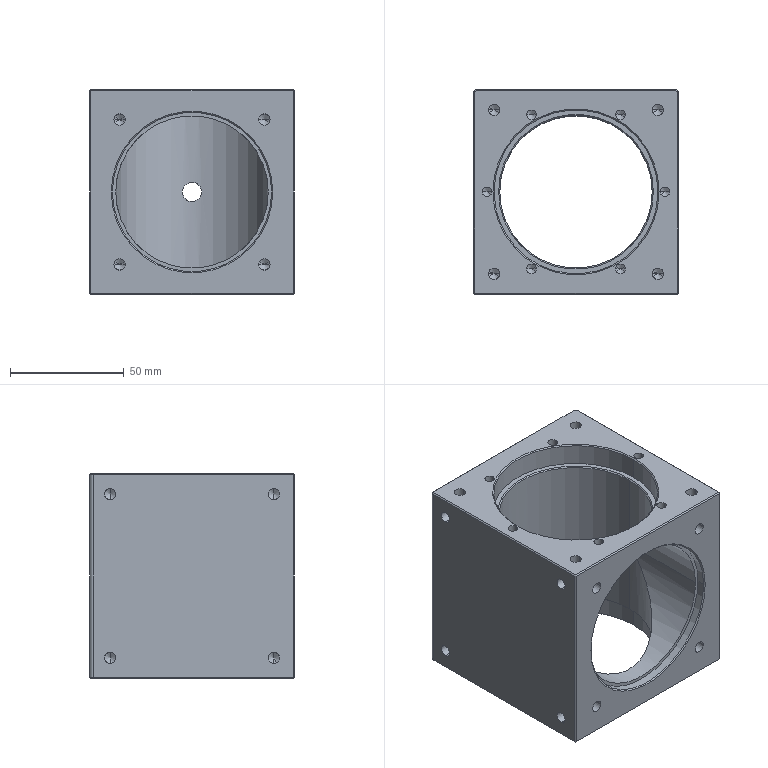NC program | NX | posted with a generic post | part box 90 x 90 x 90 mm
Whole program:
N10 G17 G21 G94 G90
(DRILLING_COPY_1_COPY_1_COPY_COPY , TOOL : D6A45)
N12 T07 M6
N14 G54
N16 G17 G0 G90 X0. Y0. B0. C0. S5000 M3
N18 G43 Z30. H7
N20 G94 G81 G98 Z-1. F250. R3.
N22 X-19.55 Y33.862
N24 X-36. Y36.
N26 X-39.1 Y0.
N28 X-36. Y-36.
N30 X-19.55 Y-33.862
N32 X19.55
N34 X36. Y-36.
N36 X39.1 Y0.
N38 X36. Y36.
N40 X19.55 Y33.862
N42 G80
N44 G0 X19.55 Y33.862 Z30.
N46 M5
(DRILLING_COPY_1_COPY_COPY_COPY_COPY_COPY_1_COPY_1 , TOOL : 5.0ZT)
N48 T15 M6
N50 G54
N52 G17 G0 G90 X-36. Y36. B0. C0. S2000 M3
N54 G43 Z30. H15
N56 G94 G83 G98 Z-10.234 F150. Q2. R3.
N58 Y-36. Z-12.002
N60 X36.
N62 Y36. Z-10.234
N64 G80
N66 G0 X36. Y36. Z30.
N68 M5
(DRILLING_COPY_1_COPY_COPY_COPY_COPY_COPY_1_COPY_COPY , TOOL : 4.2ZT)
N70 T14 M6
N72 G54
N74 G17 G0 G90 X-39.1 Y0. B0. C0. S2000 M3
N76 G43 Z30. H14
N78 G94 G83 G98 Z-15.262 F150. Q2. R3.
N80 X-19.55 Y33.862
N82 X19.55
N84 X39.1 Y0.
N86 X19.55 Y-33.862
N88 X-19.55
N90 G80
N92 G0 X-19.55 Y-33.862 Z30.
N94 M5
(DRILLING_COPY_1_COPY_COPY_COPY_COPY_COPY_COPY_COPY , TOOL : 9.0ZT)
N96 T09 M6
N98 G54
N100 G17 G0 G90 X0. Y0. B0. C0. S1200 M3
N102 G43 Z30. H9
N104 G94 G83 G98 Z-49.704 F150. Q2. R3.
N106 G80
N108 G0 X0. Y0. Z30.
N110 M5
(HOLE_MILLING_COPY_1_COPY , TOOL : D10)
N112 T10 M6
N114 G54
N116 G17 G0 G90 X0. Y0. B0. C0. S9500 M3
N118 G43 Z30. H10
N120 Z0.5
N122 G94 G3 X-1.25 Y1.25 R1.25 F2200.
N124 X-2.5 Y0. R1.25
N126 X-2.5 Y0. Z-0.5 I2.5 J0.
N128 X-2.5 Y0. Z-1.5 I2.5 J0.
N130 X-2.5 Y0. Z-2.5 I2.5 J0.
N132 X-2.5 Y0. Z-3.5 I2.5 J0.
N134 X-2.5 Y0. Z-4.5 I2.5 J0.
N136 X-2.5 Y0. Z-5.5 I2.5 J0.
N138 X-2.5 Y0. Z-6.5 I2.5 J0.
N140 X-2.5 Y0. Z-7.5 I2.5 J0.
N142 X-2.5 Y0. Z-8.5 I2.5 J0.
N144 X-2.5 Y0. Z-9.5 I2.5 J0.
N146 X0.099 Y-2.678 R2.68
N148 X2.987 Y-0.165 R2.819
N150 X0.334 Y3.217 R3.076
N152 X-3.461 Y0.383 R3.39
N154 X-0.578 Y-3.681 R3.568
N156 X3.919 Y-0.654 R3.881
N158 X0.874 Y4.126 R4.06
N160 X-4.357 Y0.976 R4.373
N162 X-1.22 Y-4.548 R4.551
N164 X4.769 Y-1.349 R4.865
N166 X1.615 Y4.943 R5.043
N168 X-5.152 Y1.769 R5.356
N170 X-2.058 Y-5.307 R5.534
N172 X5.502 Y-2.235 R5.847
N174 X2.544 Y5.635 R6.025
N176 X-5.815 Y2.744 R6.339
N178 X-3.072 Y-5.925 R6.517
N180 X6.087 Y-3.294 R6.83
N182 X3.64 Y6.172 R7.008
N184 X-6.315 Y3.882 R7.322
N186 X-4.243 Y-6.374 R7.5
N188 X6.495 Y-4.503 R7.813
N190 X4.879 Y6.526 R7.991
N192 X-6.625 Y5.156 R8.304
N194 X-5.543 Y-6.627 R8.482
N196 X6.701 Y-5.836 R8.796
N198 X6.232 Y6.673 R8.974
N200 X-6.721 Y6.539 R9.287
N202 X-6.943 Y-6.662 R9.465
N204 X6.684 Y-7.26 R9.778
N206 X7.67 Y6.592 R9.956
N208 X-6.586 Y7.997 R10.269
N210 X-8.409 Y-6.461 R10.447
N212 X6.426 Y-8.743 R10.761
N214 X9.156 Y6.268 R10.939
N216 X-6.204 Y9.495 R11.252
N218 X-9.906 Y-6.012 R11.43
N220 X5.917 Y-10.248 R11.743
N222 X10.654 Y5.691 R11.921
N224 X-5.565 Y10.997 R12.235
N226 X-11.395 Y-5.305 R12.413
N228 X5.148 Y-11.736 R12.726
N230 X12.125 Y4.854 R12.904
N232 X-4.666 Y12.462 R13.217
N234 X-12.839 Y-4.338 R13.395
N236 X4.119 Y-13.169 R13.708
N238 X13.531 Y3.758 R13.886
N240 X-3.508 Y13.852 R14.2
N242 X-14.197 Y-3.114 R14.378
N244 X2.834 Y-14.507 R14.691
N246 X14.832 Y2.408 R14.869
N248 X-2.098 Y15.127 R15.182
N250 X-15.43 Y-1.642 R15.36
N252 X1.302 Y-15.709 R15.673
N254 X15.987 Y0.816 R15.851
N256 X-0.448 Y16.248 R16.165
N258 X-16.499 Y0.066 R16.343
N260 X-0.461 Y-16.739 R16.656
N262 X16.961 Y-1.002 R16.834
N264 X1.423 Y17.178 R17.147
N266 X-17.369 Y1.989 R17.325
N268 X-2.435 Y-17.56 R17.638
N270 X17.717 Y-3.023 R17.816
N272 X3.493 Y17.881 R18.13
N274 X-18.003 Y4.102 R18.308
N276 X-4.593 Y-18.138 R18.621
N278 X18.222 Y-5.221 R18.799
N280 X5.732 Y18.326 R19.112
N282 X-18.372 Y6.377 R19.29
N284 X-6.905 Y-18.443 R19.603
N286 X18.448 Y-7.564 R19.781
N288 X8.108 Y18.484 R20.095
N290 X-18.447 Y8.778 R20.273
N292 X-9.336 Y-18.448 R20.586
N294 X18.368 Y-10.015 R20.764
N296 X10.583 Y18.331 R21.077
N298 X-18.207 Y11.269 R21.255
N300 X-11.846 Y-18.131 R21.568
N302 X17.962 Y-12.535 R21.746
N304 X13.117 Y17.847 R22.06
N306 X-17.632 Y13.807 R22.238
N308 X-14.393 Y-17.476 R22.551
N310 X17.215 Y-15.08 R22.729
N312 X15.667 Y17.018 R23.042
N314 X-16.71 Y16.348 R23.22
N316 X-16.932 Y-16.472 R23.533
N318 X16.117 Y-17.605 R23.711
N320 X18.185 Y15.837 R24.025
N322 X-15.435 Y18.845 R24.202
N324 X-19.417 Y-15.113 R24.516
N326 X14.664 Y-20.063 R24.694
N328 X20.624 Y14.3 R25.007
N330 X-13.805 Y21.251 R25.185
N332 X-21.799 Y-13.4 R25.498
N334 X12.859 Y-22.405 R25.676
N336 X22.936 Y12.412 R25.989
N338 X-11.827 Y23.518 R26.167
N340 X-24.029 Y-11.34 R26.481
N342 X10.711 Y-24.583 R26.659
N344 X25.072 Y10.183 R26.972
N346 X-9.513 Y25.596 R27.15
N348 X-26.06 Y-8.946 R27.463
N350 X8.235 Y-26.55 R27.641
N352 X26.986 Y7.631 R27.954
N354 X-6.881 Y27.44 R28.132
N356 X-27.844 Y-6.24 R28.446
N358 X5.453 Y-28.259 R28.624
N360 X28.63 Y4.778 R28.937
N362 X-3.955 Y29.003 R29.115
N364 X-29.338 Y-3.247 R29.428
N366 X2.392 Y-29.667 R29.606
N368 X29.963 Y1.653 R29.919
N370 X-1.001 Y30.316 R30.177
N372 X-30.5 Y0. R30.328
N374 X0. Y-30.5 R30.5
N376 X-30.5 Y0. R-30.5
N378 X-15.25 Y-15.25 R15.25
N380 X0. Y0. R15.25
N382 G0 Z30.
N384 M5
(HOLE_MILLING_COPY_COPY_1_COPY , TOOL : D16)
N386 T16 M6
N388 G54
N390 G17 G0 G90 X0. Y0. B0. C0. S8500 M3
N392 G43 Z30. H16
N394 Z-10.
N396 G94 G3 X1.5 Y-1.5 R1.5 F2200.
N398 X3. Y0. R1.5
N400 X3. Y0. Z-11. I-3. J0.
N402 X3. Y0. Z-12. I-3. J0.
N404 X3. Y0. Z-13. I-3. J0.
N406 X3. Y0. Z-14. I-3. J0.
N408 X3. Y0. Z-15. I-3. J0.
N410 X3. Y0. Z-16. I-3. J0.
N412 X3. Y0. Z-17. I-3. J0.
N414 X3. Y0. Z-18. I-3. J0.
N416 X3. Y0. Z-19. I-3. J0.
N418 X3. Y0. Z-20. I-3. J0.
N420 X3. Y0. Z-21. I-3. J0.
N422 X3. Y0. Z-22. I-3. J0.
N424 X3. Y0. Z-23. I-3. J0.
N426 X3. Y0. Z-24. I-3. J0.
N428 X3. Y0. Z-25. I-3. J0.
N430 X3. Y0. Z-26. I-3. J0.
N432 X3. Y0. Z-27. I-3. J0.
N434 X3. Y0. Z-28. I-3. J0.
N436 X0. Y-3. Z-28.75 R-3.
N438 X3.177 Y0.106 R3.178
N440 X0.146 Y3.49 R3.322
N442 X-3.726 Y0.302 R3.579
N444 X-0.334 Y-3.973 R3.894
N446 X4.201 Y-0.509 R4.073
N448 X0.561 Y4.445 R4.388
N450 X-4.664 Y0.756 R4.567
N452 X-0.829 Y-4.904 R4.881
N454 X5.113 Y-1.043 R5.06
N456 X1.137 Y5.347 R5.375
N458 X-5.545 Y1.369 R5.554
N460 X-1.482 Y-5.773 R5.868
N462 X5.958 Y-1.733 R6.047
N464 X1.865 Y6.178 R6.362
N466 X-6.35 Y2.133 R6.541
N468 X-2.285 Y-6.56 R6.855
N470 X6.718 Y-2.569 R7.034
N472 X2.739 Y6.918 R7.349
N474 X-7.059 Y3.04 R7.528
N476 X-3.227 Y-7.247 R7.842
N478 X7.372 Y-3.543 R8.021
N480 X3.747 Y7.548 R8.336
N482 X-7.654 Y4.077 R8.515
N484 X-4.297 Y-7.817 R8.829
N486 X7.904 Y-4.64 R9.008
N488 X4.876 Y8.052 R9.323
N490 X-8.12 Y5.232 R9.501
N492 X-5.482 Y-8.251 R9.816
N494 X8.299 Y-5.849 R9.995
N496 X6.113 Y8.414 R10.309
N498 X-8.439 Y6.489 R10.488
N500 X-6.766 Y-8.537 R10.803
N502 X8.54 Y-7.152 R10.982
N504 X7.44 Y8.62 R11.296
N506 X-8.6 Y7.833 R11.475
N508 X-8.132 Y-8.66 R11.79
N510 X8.617 Y-8.531 R11.968
N512 X8.84 Y8.657 R12.283
N514 X-8.59 Y9.244 R12.462
N516 X-9.562 Y-8.609 R12.776
N518 X8.518 Y-9.97 R12.955
N520 X10.294 Y8.516 R13.27
N522 X-8.399 Y10.704 R13.448
N524 X-11.035 Y-8.376 R13.763
N526 X8.234 Y-11.446 R13.942
N528 X11.781 Y8.188 R14.256
N530 X-8.02 Y12.191 R14.435
N532 X-12.53 Y-7.952 R14.75
N534 X7.758 Y-12.938 R14.929
N536 X13.279 Y7.667 R15.243
N538 X-7.447 Y13.684 R15.422
N540 X-14.026 Y-7.332 R15.736
N542 X7.087 Y-14.426 R15.915
N544 X14.767 Y6.949 R16.23
N546 X-6.677 Y15.161 R16.409
N548 X-15.5 Y-6.515 R16.723
N550 X6.218 Y-15.886 R16.902
N552 X16.221 Y6.033 R17.217
N554 X-5.71 Y16.598 R17.395
N556 X-16.929 Y-5.501 R17.71
N558 X5.152 Y-17.295 R17.889
N560 X17.619 Y4.919 R18.203
N562 X-4.546 Y17.974 R18.382
N564 X-18.29 Y-4.29 R18.697
N566 X3.892 Y-18.631 R18.875
N568 X18.938 Y3.613 R19.19
N570 X-3.191 Y19.264 R19.369
N572 X-19.561 Y-2.889 R19.683
N574 X2.443 Y-19.87 R19.862
N576 X20.156 Y2.118 R20.177
N578 X-1.65 Y20.446 R20.355
N580 X-20.719 Y-1.304 R20.67
N582 X0.813 Y-20.991 R20.849
N584 X21.249 Y0.445 R21.163
N586 X0.066 Y21.5 R21.342
N588 X-21.742 Y0.455 R21.657
N590 X-0.987 Y-21.971 R21.836
N592 X22.196 Y-1.396 R22.15
N594 X1.948 Y22.402 R22.329
N596 X-22.609 Y2.376 R22.643
N598 X-2.946 Y-22.79 R22.822
N600 X22.977 Y-3.393 R23.137
N602 X3.98 Y23.133 R23.316
N604 X-23.3 Y4.445 R23.63
N606 X-5.048 Y-23.429 R23.809
N608 X23.574 Y-5.529 R24.123
N610 X6.147 Y23.675 R24.302
N612 X-23.797 Y6.644 R24.617
N614 X-7.076 Y-24.012 R24.875
N616 X23.967 Y-7.787 R25.028
N618 X7.787 Y23.967 R25.2
N620 X23.967 Y-7.787 R-25.2
N622 X15.877 Y8.09 R12.6
N624 X0. Y0. R12.6
N626 X1.5 Y-1.5 R1.5
N628 X3. Y0. R1.5
N630 X3. Y0. Z-29.75 I-3. J0.
N632 X3. Y0. Z-30.75 I-3. J0.
N634 X3. Y0. Z-31.75 I-3. J0.
N636 X3. Y0. Z-32.75 I-3. J0.
N638 X3. Y0. Z-33.75 I-3. J0.
N640 X3. Y0. Z-34.75 I-3. J0.
N642 X3. Y0. Z-35.75 I-3. J0.
N644 X3. Y0. Z-36.75 I-3. J0.
N646 X3. Y0. Z-37.75 I-3. J0.
N648 X3. Y0. Z-38.75 I-3. J0.
N650 X3. Y0. Z-39.75 I-3. J0.
N652 X3. Y0. Z-40.75 I-3. J0.
N654 X3. Y0. Z-41.75 I-3. J0.
N656 X3. Y0. Z-42.75 I-3. J0.
N658 X3. Y0. Z-43.75 I-3. J0.
N660 X3. Y0. Z-44.75 I-3. J0.
N662 X3. Y0. Z-45.75 I-3. J0.
N664 X3. Y0. Z-46.75 I-3. J0.
N666 X0. Y-3. Z-47.5 R-3.
N668 X3.177 Y0.106 R3.178
N670 X0.146 Y3.49 R3.322
N672 X-3.726 Y0.302 R3.579
N674 X-0.334 Y-3.973 R3.894
N676 X4.201 Y-0.509 R4.073
N678 X0.561 Y4.445 R4.388
N680 X-4.664 Y0.756 R4.567
N682 X-0.829 Y-4.904 R4.881
N684 X5.113 Y-1.043 R5.06
N686 X1.137 Y5.347 R5.375
N688 X-5.545 Y1.369 R5.554
N690 X-1.482 Y-5.773 R5.868
N692 X5.958 Y-1.733 R6.047
N694 X1.865 Y6.178 R6.362
N696 X-6.35 Y2.133 R6.541
N698 X-2.285 Y-6.56 R6.855
N700 X6.718 Y-2.569 R7.034
N702 X2.739 Y6.918 R7.349
N704 X-7.059 Y3.04 R7.528
N706 X-3.227 Y-7.247 R7.842
N708 X7.372 Y-3.543 R8.021
N710 X3.747 Y7.548 R8.336
N712 X-7.654 Y4.077 R8.515
N714 X-4.297 Y-7.817 R8.829
N716 X7.904 Y-4.64 R9.008
N718 X4.876 Y8.052 R9.323
N720 X-8.12 Y5.232 R9.501
N722 X-5.482 Y-8.251 R9.816
N724 X8.299 Y-5.849 R9.995
N726 X6.113 Y8.414 R10.309
N728 X-8.439 Y6.489 R10.488
N730 X-6.766 Y-8.537 R10.803
N732 X8.54 Y-7.152 R10.982
N734 X7.44 Y8.62 R11.296
N736 X-8.6 Y7.833 R11.475
N738 X-8.132 Y-8.66 R11.79
N740 X8.617 Y-8.531 R11.968
N742 X8.84 Y8.657 R12.283
N744 X-8.59 Y9.244 R12.462
N746 X-9.562 Y-8.609 R12.776
N748 X8.518 Y-9.97 R12.955
N750 X10.294 Y8.516 R13.27
N752 X-8.399 Y10.704 R13.448
N754 X-11.035 Y-8.376 R13.763
N756 X8.234 Y-11.446 R13.942
N758 X11.781 Y8.188 R14.256
N760 X-8.02 Y12.191 R14.435
N762 X-12.53 Y-7.952 R14.75
N764 X7.758 Y-12.938 R14.929
N766 X13.279 Y7.667 R15.243
N768 X-7.447 Y13.684 R15.422
N770 X-14.026 Y-7.332 R15.736
N772 X7.087 Y-14.426 R15.915
N774 X14.767 Y6.949 R16.23
N776 X-6.677 Y15.161 R16.409
N778 X-15.5 Y-6.515 R16.723
N780 X6.218 Y-15.886 R16.902
N782 X16.221 Y6.033 R17.217
N784 X-5.71 Y16.598 R17.395
N786 X-16.929 Y-5.501 R17.71
N788 X5.152 Y-17.295 R17.889
N790 X17.619 Y4.919 R18.203
N792 X-4.546 Y17.974 R18.382
N794 X-18.29 Y-4.29 R18.697
N796 X3.892 Y-18.631 R18.875
N798 X18.938 Y3.613 R19.19
N800 X-3.191 Y19.264 R19.369
N802 X-19.561 Y-2.889 R19.683
N804 X2.443 Y-19.87 R19.862
N806 X20.156 Y2.118 R20.177
N808 X-1.65 Y20.446 R20.355
N810 X-20.719 Y-1.304 R20.67
N812 X0.813 Y-20.991 R20.849
N814 X21.249 Y0.445 R21.163
N816 X0.066 Y21.5 R21.342
N818 X-21.742 Y0.455 R21.657
N820 X-0.987 Y-21.971 R21.836
N822 X22.196 Y-1.396 R22.15
N824 X1.948 Y22.402 R22.329
N826 X-22.609 Y2.376 R22.643
N828 X-2.946 Y-22.79 R22.822
N830 X22.977 Y-3.393 R23.137
N832 X3.98 Y23.133 R23.316
N834 X-23.3 Y4.445 R23.63
N836 X-5.048 Y-23.429 R23.809
N838 X23.574 Y-5.529 R24.123
N840 X6.147 Y23.675 R24.302
N842 X-23.797 Y6.644 R24.617
N844 X-7.076 Y-24.012 R24.875
N846 X23.967 Y-7.787 R25.028
N848 X7.787 Y23.967 R25.2
N850 X23.967 Y-7.787 R-25.2
N852 X15.877 Y8.09 R12.6
N854 X0. Y0. R12.6
N856 G0 Z30.
N858 M5
(HOLE_MILLING_COPY_COPY_COPY_COPY , TOOL : D12JING)
N860 T12 M6
N862 G54
N864 G17 G0 G90 X23.779 Y-3.247 B0. C0. S8000 M3
N866 G43 Z30. H12
N868 Z-28.5
N870 G94 G3 X27.5 Y0. R3.277 F1000.
N872 X0. Y27.5 R27.5
N874 X27.5 Y0. R-27.5
N876 X23.779 Y3.247 R3.277
N878 G0 Y-3.247 Z-47.5
N880 G3 X27.5 Y0. R3.277
N882 X0. Y27.5 R27.5
N884 X27.5 Y0. R-27.5
N886 X23.779 Y3.247 R3.277
N888 G0 Z30.
N890 M5
(ZLEVEL_PROFILE_1_COPY_1_COPY_COPY_COPY , TOOL : D6A45)
N892 T07 M6
N894 G54
N896 G17 G0 G90 X-19.55 Y34.503 B0. C0. S9500 M3
N898 G43 Z30. H7
N900 Z1.
N902 G94 G1 Z-1.5 F1000.
N904 G3 X-20.191 Y33.862 R0.641
N906 X-19.55 Y34.503 R-0.641
N908 X-20.07 Y34.203 R0.6
N910 G1 Z-0.5
N912 G0 Z30.
N914 X-36. Y37.041
N916 Z1.
N918 G1 Z-1.5
N920 G3 X-37.041 Y36. R1.041
N922 X-36. Y37.041 R-1.041
N924 X-36.52 Y36.741 R0.6
N926 G1 Z-0.5
N928 G0 Z30.
N930 X1.049 Y33.825
N932 Z-0.5
N934 G1 Z-1.5
N936 X0.52 Y34.741
N938 G3 X0. Y35.041 R0.6
N940 X-35.041 Y0. R35.041
N942 X0. Y35.041 R-35.041
N944 X-0.52 Y34.741 R0.6
N946 G1 X-1.049 Y33.825
N948 Z-0.5
N950 G0 Z30.
N952 X36. Y37.041
N954 Z1.
N956 G1 Z-1.5
N958 G3 X34.959 Y36. R1.041
N960 X36. Y37.041 R-1.041
N962 X35.48 Y36.741 R0.6
N964 G1 Z-0.5
N966 G0 Z30.
N968 X-19.55 Y-34.503
N970 Z1.
N972 G1 Z-1.5
N974 G3 X-18.909 Y-33.862 R0.641
N976 X-19.55 Y-34.503 R-0.641
N978 X-19.03 Y-34.203 R0.6
N980 G1 Z-0.5
N982 G0 Z30.
N984 X36. Y-37.041
N986 Z1.
N988 G1 Z-1.5
N990 G3 X37.041 Y-36. R1.041
N992 X36. Y-37.041 R-1.041
N994 X36.52 Y-36.741 R0.6
N996 G1 Z-0.5
N998 G0 Z30.
N1000 X19.55 Y34.503
N1002 Z1.
N1004 G1 Z-1.5
N1006 G3 X18.909 Y33.862 R0.641
N1008 X19.55 Y34.503 R-0.641
N1010 X19.03 Y34.203 R0.6
N1012 G1 Z-0.5
N1014 G0 Z30.
N1016 X19.55 Y-34.503
N1018 Z1.
N1020 G1 Z-1.5
N1022 G3 X20.191 Y-33.862 R0.641
N1024 X19.55 Y-34.503 R-0.641
N1026 X20.07 Y-34.203 R0.6
N1028 G1 Z-0.5
N1030 G0 Z30.
N1032 X-36. Y-37.041
N1034 Z1.
N1036 G1 Z-1.5
N1038 G3 X-34.959 Y-36. R1.041
N1040 X-36. Y-37.041 R-1.041
N1042 X-35.48 Y-36.741 R0.6
N1044 G1 Z-0.5
N1046 G0 Z30.
N1048 X39.741 Y0.
N1050 Z1.
N1052 G1 Z-1.5
N1054 G3 X39.1 Y0.641 R0.641
N1056 X39.741 Y0. R-0.641
N1058 X39.441 Y0.52 R0.6
N1060 G1 Z-0.5
N1062 G0 Z30.
N1064 X-39.741 Y0.
N1066 Z1.
N1068 G1 Z-1.5
N1070 Y-0.005
N1072 G3 X-39.095 Y-0.641 R0.641
N1074 X-39.741 Y0. R-0.641
N1076 X-39.441 Y-0.52 R0.6
N1078 G1 Z-0.5
N1080 G0 Z30.
N1082 X-46.987 Y-45.441
N1084 Z-0.5
N1086 G1 Z-1.5
N1088 X-46.259 Y-45.02
N1090 G3 X-45.959 Y-44.501 R0.6
N1092 G1 Y43.5
N1094 G2 X-43.5 Y45.959 R2.459
N1096 G1 X43.5
N1098 G2 X45.959 Y43.5 R2.459
N1100 G1 Y-44.501
N1102 G2 X44.501 Y-45.959 R1.458
N1104 G1 X-44.501
N1106 G2 X-45.959 Y-44.501 R1.458
N1108 G3 X-46.259 Y-43.981 R0.6
N1110 G1 X-47.159 Y-43.462
N1112 Z-0.5
N1114 G0 Z30.
N1116 M5
N1118 M2